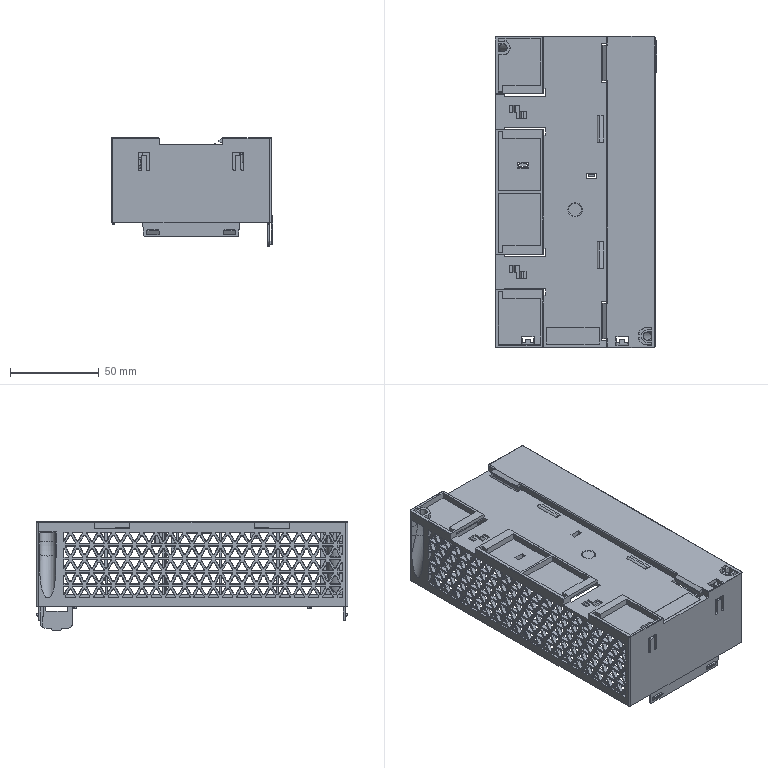Part | Creo | 1 solid | 3981 faces | volume 77601 mm3 | spline 1578 | plane 1336 | cone 847 | cylinder 163 | other 27 | torus 20 | sphere 10 | commonest cylinder face diameters 0.402 x58 1.005 x41 0.603 x18 2.01 x12 5.226 x4 6.03 x4